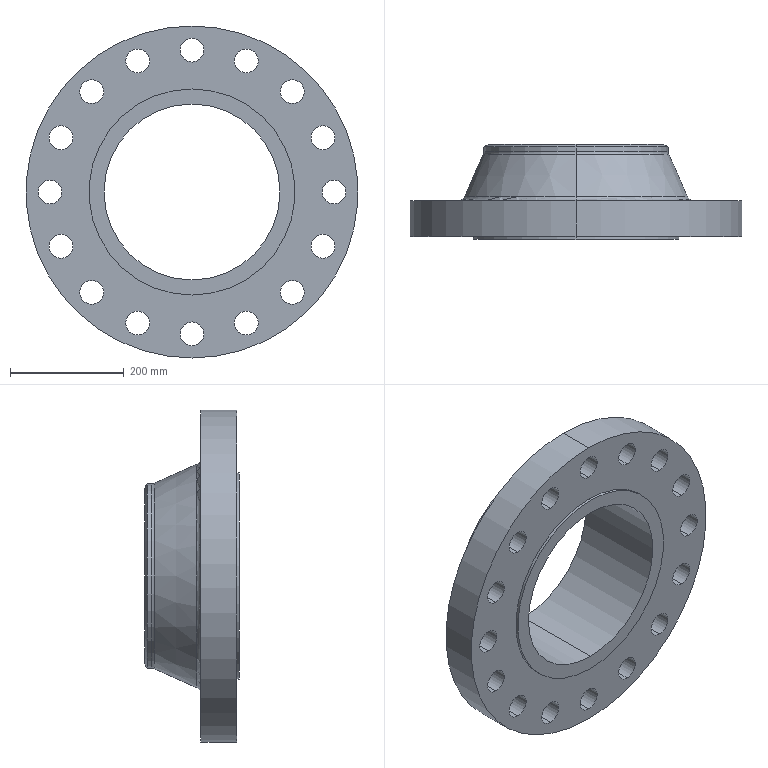Part | NX | features BREP 1, Resize Face 1 | 1 solid | 51 faces | box 585 x 167.113 x 585 mm | volume 13392548 mm3 | cylinder 40 | cone 4 | torus 4 | plane 3 | commonest cylinder face diameters 42 x32 310 x2 325 x2 363 x2 585 x2